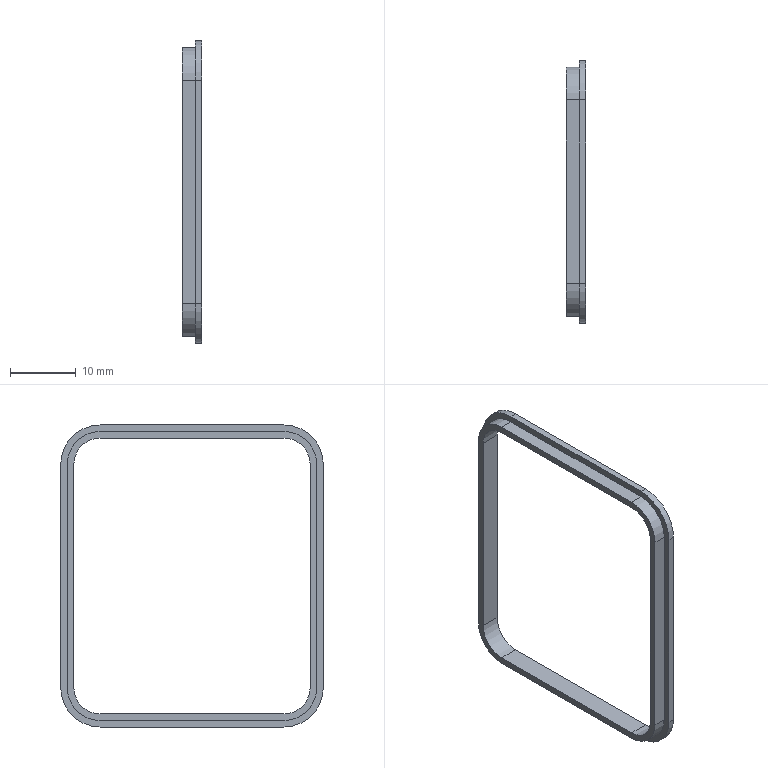Part | STEP file | 1-31.7 | 1 solid | 27 faces | box 3 x 40 x 46 mm | volume 615.381 mm3 | plane 15 | cylinder 12 | commonest cylinder face diameters 8 x4 10 x4 12 x4